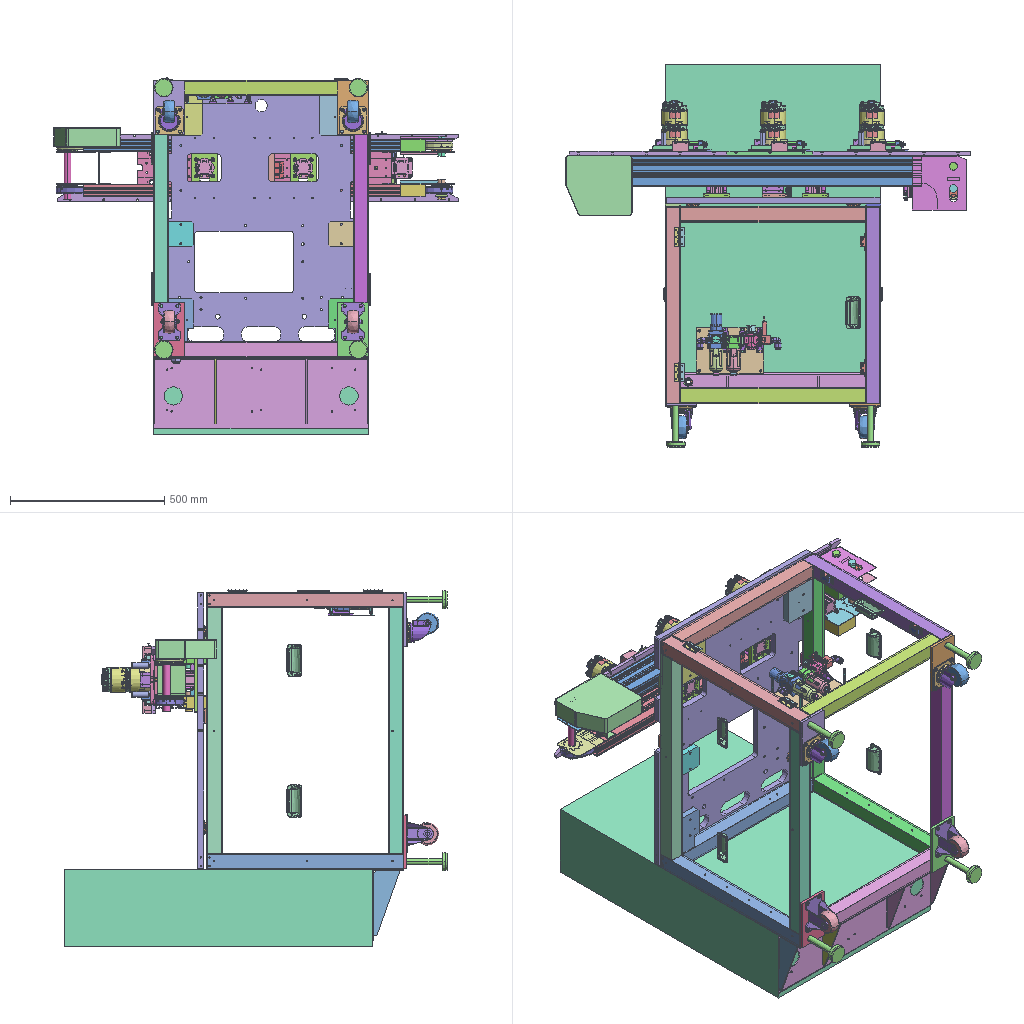Assembly | STEP file | 115 different items | 496 placed | box 1312 x 1242 x 1158 mm
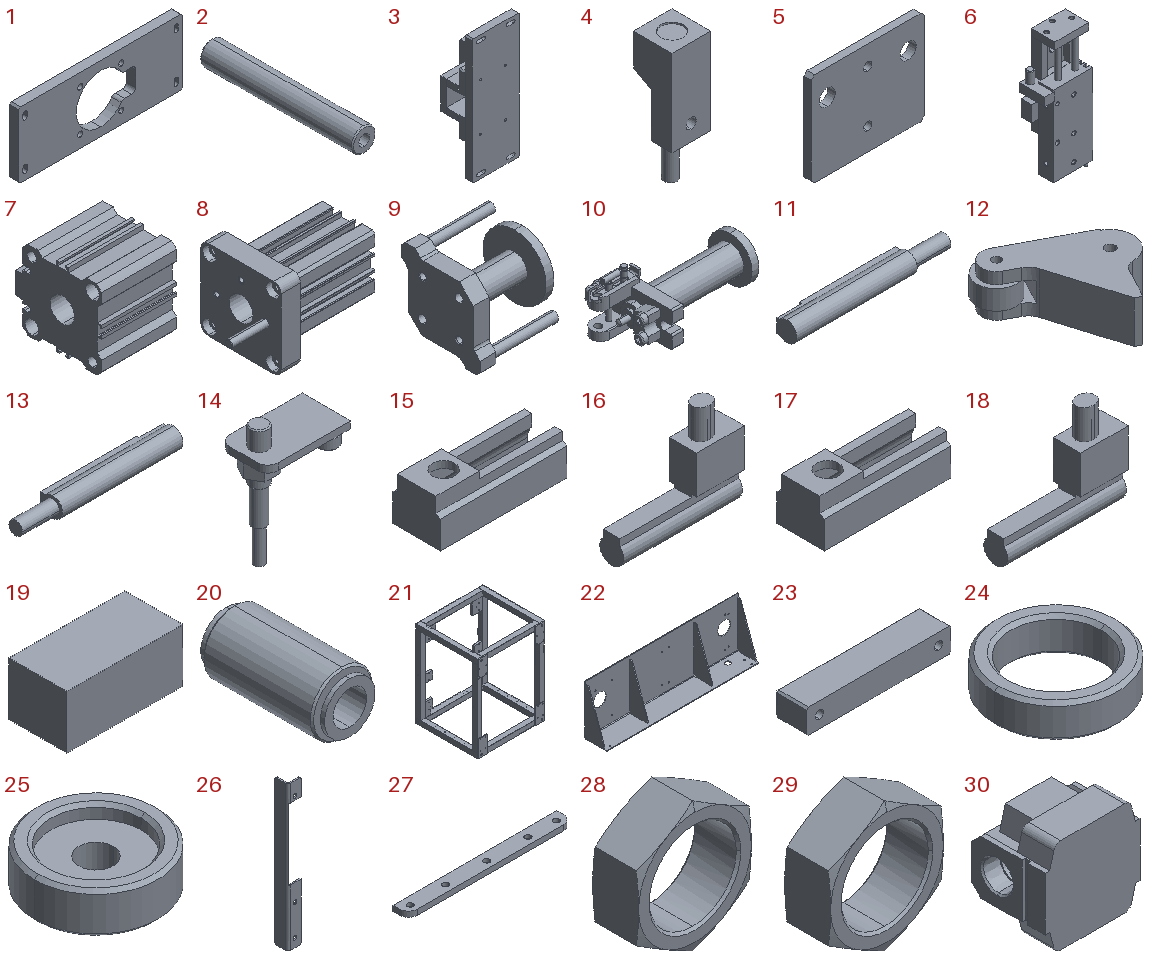Parts list (item | name | quantity | parent item | size | volume):
1 | 1105-104P042 | x2 | in 1105 brake cylinder | 211 x 12 x 85 mm | 165704 mm3
2 | 1105-104P043 | x12 | in 1105 brake cylinder | 11 x 71 x 11 mm | 6130 mm3
3 | 1105-104P044 | x1 | in 1105WWTCDQMB40-10-A93L_0_0_0_ | 79.5 x 92 x 211 mm | 345527 mm3
4 | 1105WWAAPS4-12M-Z-R-1-001 | x3 | in PN_0002 in-position detection Default | 12 x 12 x 37 mm | 2919 mm3
5 | 1105WWASensor BKT | x3 | in PN_0002 in-position detection Default | 35 x 2.3 x 29 mm | 2217 mm3
6 | 1105WWMXQ12-40CSP-M9NL(35)527 | x1 | in 1105WWNACCTV松Product-00527 | 56.1 x 30 x 145 mm | 123315 mm3
7 | 1105WWT1_1 | x1 | in 1105WWTCDQMB40-10-A93L_0_0_0_ | 49.5 x 57 x 52 mm | 94485 mm3
8 | 1105WWT1_2 | x3 | - | 120 x 67 x 67 mm | 176582 mm3
9 | 1105WWT2_1 | x1 | in 1105WWTCDQMB40-10-A93L_0_0_0_ | 51.75 x 50 x 50 mm | 33168 mm3
10 | 1105WWT2_2 | x3 | - | 97 x 42.5 x 39.25 mm | 37426 mm3
11 | 1105WWT3 | x1 | in 1105WWTCDQMB40-10-A93L_0_0_0_ | 32 x 4.5 x 4 mm | 389.357 mm3
12 | 1105WWT3_1 | x3 | - | 33.665 x 38.307 x 13 mm | 6665 mm3
13 | 1105WWT4 | x1 | in 1105WWTCDQMB40-10-A93L_0_0_0_ | 32 x 4.5 x 4 mm | 389.357 mm3
14 | 1105WWT4_1 | x3 | - | 24.119 x 14.25 x 35 mm | 1315 mm3
15 | 1105WWT5_1 | x3 | - | 16.5 x 6.2 x 5.9 mm | 230.408 mm3
16 | 1105WWT6_1 | x3 | - | 20 x 4.6 x 16.5 mm | 577.001 mm3
17 | 1105WWT7_1 | x3 | - | 16.5 x 6.2 x 5.9 mm | 230.408 mm3
18 | 1105WWT8_1 | x3 | - | 20 x 4.6 x 16.5 mm | 577.001 mm3
19 | 1105WW撞块-002_デフォルト | x3 | in 1105WW442_デフォルト | 30 x 15 x 13.8 mm | 6210 mm3
20 | 1_4 | x1 | in KQ2E12-00 | 22 x 44 x 22 mm | 10940 mm3
21 | 227H056111 Footstool Default | x1 | in 18 | 700 x 656 x 900 mm | 6881693 mm3
22 | 227H056114 BKT Default | x1 | in 18 | 700 x 100 x 230 mm | 887594 mm3
23 | 229H151426 Default | x6 | in PN_0018 Default | 80 x 17.5 x 13.5 mm | 17874 mm3
24 | 229H151427 Default | x6 | in PN_0018 Default | 18 x 18 x 5 mm | 563.602 mm3
25 | 229H151428 Default | x6 | in PN_0018 Default | 18 x 18 x 6 mm | 1155 mm3
26 | 229H151431 Default | x3 | in PN_0018 Default | 15 x 15 x 165 mm | 5074 mm3
27 | 229H151433 Default | x3 | in PN_0018 Default | 185 x 17.5 x 6 mm | 18413 mm3
28 | 2_4 | x1 | in KQ2E12-00 | 27 x 11 x 31.177 mm | 3125 mm3
29 | 3 | x1 | in KQ2E12-00 | 27 x 11 x 31.177 mm | 3125 mm3
30 | AFM30-03_AFM3022A Body_30 | x1 | in AFM30-03_AFM30-03 | 53 x 41 x 53 mm | 82463 mm3
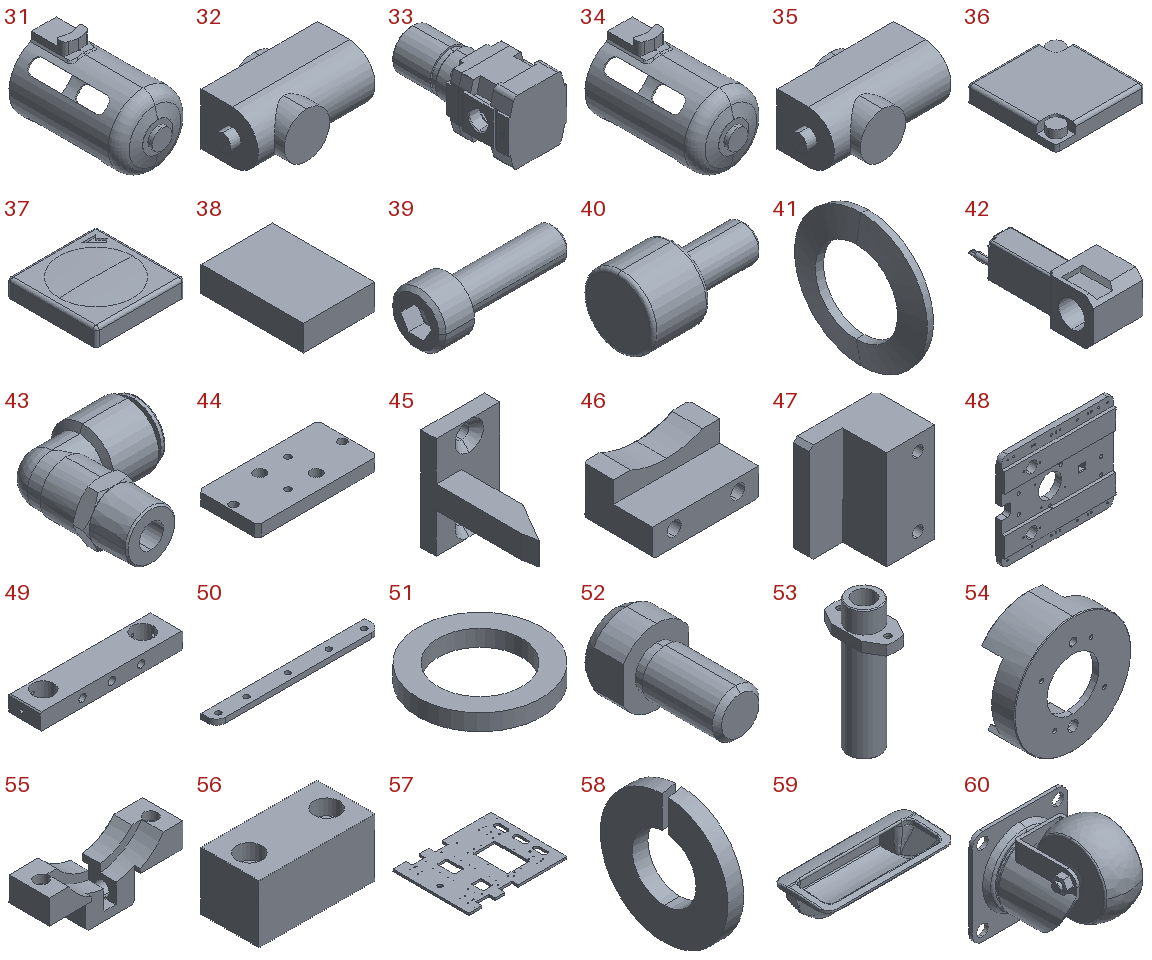31 | AFM30-03_AFM3022A Bowl_30 | x1 | in AFM30-03_AFM3022A Bowl Assy_30 | 45.5 x 76.9 x 53.25 mm | 11501 mm3
32 | AFM30-03_AFM3022A Drain_30 | x1 | in AFM30-03_AFM3022A Bowl Assy_30 | 19.5 x 11.1 x 8 mm | 1266 mm3
33 | AW30-03E_AW3020A Body_30 | x1 | in AW30-03E_AW30-03E | 53 x 113 x 57 mm | 188440 mm3
34 | AW30-03E_AW3020A Bowl_30 | x1 | in AW30-03E_AW3020A Bowl Assy_30 | 45.5 x 76.9 x 53.25 mm | 11501 mm3
35 | AW30-03E_AW3020A Drain_30 | x1 | in AW30-03E_AW3020A Bowl Assy_30 | 19.5 x 11.1 x 8 mm | 1266 mm3
36 | AW30-03E_AW3020A Gauge_30 | x1 | in AW30-03E_AW30-03E | 28 x 28 x 5.1 mm | 3850 mm3
37 | AW30-03E_AW3020A Gauge_30-E | x1 | in AW30-03E_AW30-03E | 28 x 28 x 5.8 mm | 4343 mm3
38 | BOX111 Default | x1 | in 18 | 700 x 1000 x 250 mm | 175000000 mm3
39 | CB6-20_デフォルト | x24 | in CB6-20_CW6_デフォルト, CB6-20_SW6_W6_デフォルト | 26 x 10 x 10 mm | 957.413 mm3
40 | CFFANG5-10_デフォルト | x3 | in PN_0018 Default | 18 x 10 x 10 mm | 819.54 mm3
41 | CW6 Default | x12 | in CB6-20_CW6_デフォルト | 0.95 x 10.5 x 10.5 mm | 31.798 mm3
42 | IS1000E-3003-X202_IS1000E3035GA Body_30 | x1 | in IS1000E-3003-X202_IS1000E-3003-X202 | 32 x 90.5 x 30 mm | 34770 mm3
43 | KQ2L12-03S_KQ2L_12-03 | x2 | in KQ2L12-03S_KQ2L12-03S | 38.315 x 43.45 x 20.9 mm | 10699 mm3
44 | PN_0002 top plate Default | x1 | in 1105WWTCDQMB40-10-A93L_0_0_0_ | 100 x 50 x 10 mm | 47660 mm3
45 | PN_0002NACCTV wedge pin 527 | x1 | in 1105WWNACCTV松Product-00527 | 25 x 45.321 x 40 mm | 8429 mm3
46 | PN_0004 Default | x3 | in PN_0018 Default | 50 x 33 x 23 mm | 24275 mm3
47 | PN_0006 Default | x9 | in PN_0018 Default | 41.5 x 29.8 x 50 mm | 40902 mm3
48 | PN_0007 Default | x3 | in PN_0018 Default | 185 x 15 x 160 mm | 319731 mm3
49 | PN_0008 Default | x3 | in PN_0018 Default | 129 x 29.5 x 15 mm | 43870 mm3
50 | PN_0009 Default | x3 | in PN_0018 Default | 185 x 17.5 x 6 mm | 18511 mm3
51 | PN_0010 Default | x3 | in PN_0018 Default | 7.5 x 7.5 x 1 mm | 23.75 mm3
52 | PN_0011 Default | x3 | in PN_0018 Default | 7 x 13.2 x 8 mm | 366.094 mm3
53 | PN_0016 Default | x6 | in PN_0018 Default | 20 x 36 x 72.5 mm | 11823 mm3
54 | PN_0017 Default | x3 | in PN_0018 Default | 90 x 34.5 x 90 mm | 46936 mm3
55 | PN_0019 Default | x3 | in PN_0018 Default | 110 x 33 x 44 mm | 53876 mm3
56 | PN_0020 Default | x9 | in PN_0018 Default | 30 x 15 x 15 mm | 6285 mm3
57 | PN_0022 Base Default | x1 | in 18 | 900 x 700 x 20 mm | 9845455 mm3
58 | SW6 Default | x12 | in CB6-20_SW6_W6_デフォルト | 1.5 x 12.2 x 12.197 mm | 128.674 mm3
59 | - | x5 | in 18 | 104 x 48 x 25.005 mm | 18990 mm3
60 | SceondCJH75 | x2 | in 18 | - | -
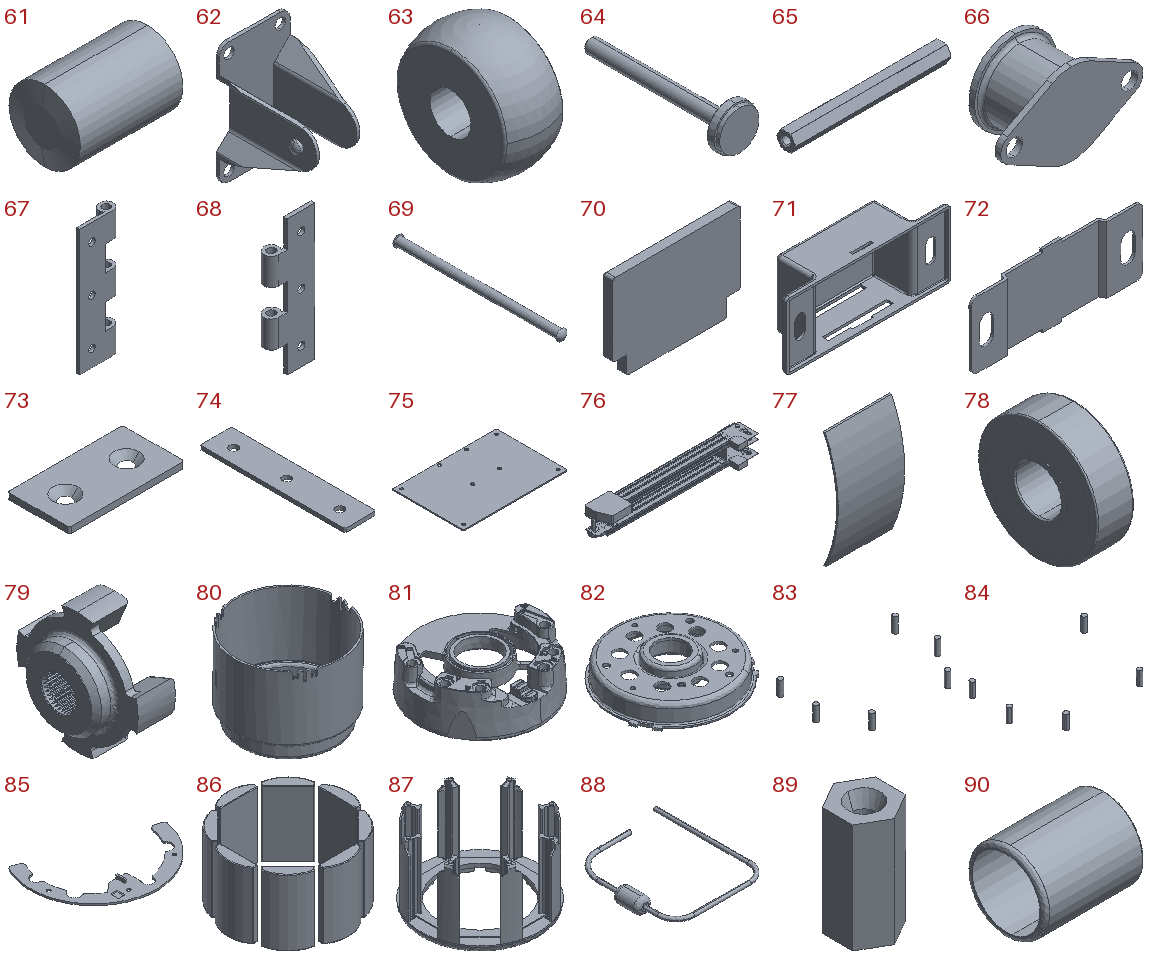61 | SceondCKH75bearing | x2 | in SceondCKH75 | 38 x 25 x 25 mm | 18231 mm3
62 | SceondCKH75fixed | x2 | in SceondCKH75 | 72 x 88.179 x 123 mm | 53019 mm3
63 | SceondCKH75wheel | x2 | in SceondCKH75 | 36 x 75 x 75 mm | 129056 mm3
64 | SceondD-B3-20-180 | x4 | in 18 | 60.3 x 210 x 60.3 mm | 105197 mm3
65 | SceondLSFB8-75 | x4 | in 18 | 75 x 9.2 x 8 mm | 3839 mm3
66 | SceondRB-45 | x4 | in 18 | 78 x 34 x 45 mm | 42765 mm3
67 | Second B-1027-14 Pin A Part | x2 | in SceondB-1027-14 | 19.25 x 6.5 x 60 mm | 2015 mm3
68 | Second B-1027-14 Pin B Part | x2 | in SceondB-1027-14 | 19.25 x 6.5 x 60 mm | 1700 mm3
69 | Second B-1027-14 Shaft Part | x2 | in SceondB-1027-14 | 4 x 62.171 x 4 mm | 439.342 mm3
70 | Second C-100-B Work Part | x2 | in 70 | 28 x 2 x 20 mm | 1071 mm3
71 | Second C-100-B-2 Base Part | x2 | in SceondC-100-B-2 | 56.5 x 15.3 x 23 mm | 2154 mm3
72 | Second C-100-B-2 Bracket Part | x2 | in SceondC-100-B-2 | 54.5 x 2.5 x 23 mm | 897.584 mm3
73 | Second C-100-B-2 Bracket Part [2] | x2 | in 18 | 30 x 16 x 1.6 mm | 705.168 mm3
74 | Second Door Spacer PN_0025 Default | x2 | in 18 | 13 x 60 x 1.6 mm | 1201 mm3
75 | Second M80U005006A Air System BKT Default | x1 | in 18 | 220 x 150 x 2.3 mm | 75278 mm3
76 | TCSW62A-MD-145-1213-18-90W-3-SC-1014_no bracket 2090<machined> | x1 | in Tshusongxian-01_デフォルト | 1300 x 197.8 x 232.2 mm | 4651494 mm3
77 | TQ-DD-1020-BIAOQIAN-001010 | x6 | in TQ-DD-1105-TH140P_HP_K04502_MotorAssy1010_デフォルト | 20 x 4.519 x 35 mm | 361.459 mm3
78 | TQ-DD-1105-TH 6000ZZ_2_031010 Default | x6 | in TQ-DD-1105-THRotorAssy1010_デフォルト | 8 x 26 x 26 mm | 2409 mm3
79 | TQ-DD-1105-TH SAP_405441541010 Default | x6 | in TQ-DD-1105-TH140P_HP_K04502_MotorAssy1010_デフォルト | 13.9 x 30 x 30 mm | 3137 mm3
80 | TQ-DD-1105-THA140062100B_Housing1010_デフォルト | x6 | in TQ-DD-1105-THHousingAssy1010_デフォルト | 82 x 82 x 64.1 mm | 27832 mm3
81 | TQ-DD-1105-THA160078900_Mold1010_デフォルト | x6 | in TQ-DD-1105-THTerminalAssy1010_デフォルト | 79.236 x 78.917 x 27.1 mm | 21027 mm3
82 | TQ-DD-1105-THBrg.Holder(A140059500A)1010_デフォルト | x6 | in TQ-DD-1105-THBrg.HolderAssy1010_デフォルト | 79.4 x 80.57 x 17.1 mm | 12458 mm3
83 | TQ-DD-1105-THCoil1010_デフォルト | x6 | in TQ-DD-1105-THStatorAssy31010_デフォルト | 46.175 x 30.321 x 5.639 mm | 82.319 mm3
84 | TQ-DD-1105-THCoil21010_デフォルト | x6 | in TQ-DD-1105-THStatorAssy31010_デフォルト | 48.573 x 32.204 x 5.639 mm | 77.064 mm3
85 | TQ-DD-1105-THCover1010_デフォルト | x6 | in TQ-DD-1105-THTerminalAssy1010_デフォルト | 73.74 x 54.492 x 3 mm | 881.003 mm3
86 | TQ-DD-1105-THMagnet1010_デフォルト | x12 | in TQ-DD-1105-THRotorCoreAssy1010_デフォルト | 39 x 39 x 21.5 mm | 6144 mm3
87 | TQ-DD-1105-THMagnetHolder1010_デフォルト | x12 | in TQ-DD-1105-THRotor1010_デフォルト | 38.83 x 38.83 x 24.45 mm | 2757 mm3
88 | TQ-DD-1105-THNTC Thermistor1010_デフォルト | x6 | in TQ-DD-1105-THTerminalAssy1010_デフォルト | 11.725 x 13.225 x 1.8 mm | 12.894 mm3
89 | TQ-DD-1105-THNuts1010_デフォルト | x36 | in TQ-DD-1105-THTerminalAssy1010_デフォルト | 6 x 6.928 x 12.4 mm | 316.696 mm3
90 | TQ-DD-1105-THRotor cover1010_デフォルト | x6 | in TQ-DD-1105-THRotorCoreAssy1010_デフォルト | 48.9 x 39.4 x 39.4 mm | 1331 mm3
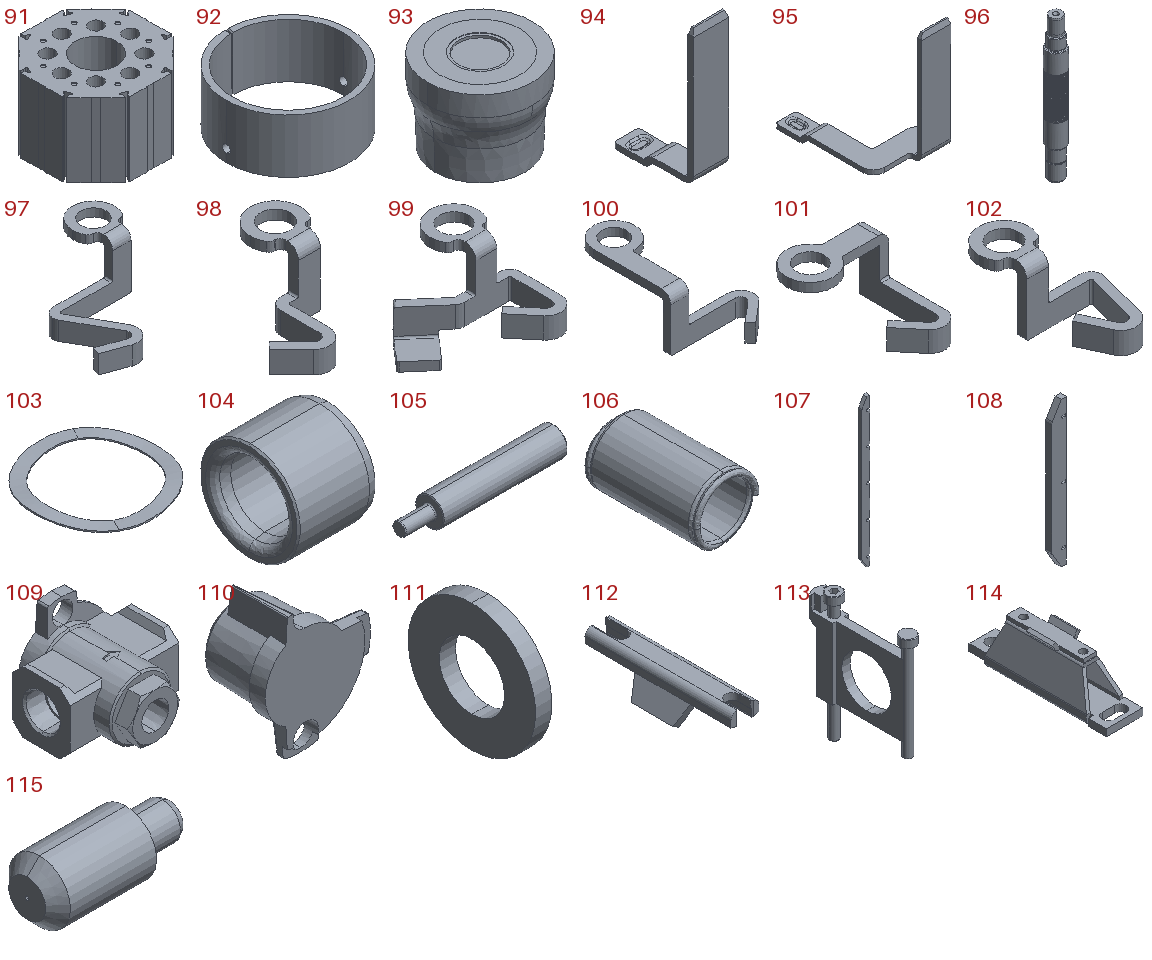91 | TQ-DD-1105-THRotorCore1010_デフォルト | x12 | in TQ-DD-1105-THRotor1010_デフォルト | 31.8 x 31.8 x 21.5 mm | 12871 mm3
92 | TQ-DD-1105-THSHIELD1010_デフォルト | x6 | in TQ-DD-1105-THTerminalAssy1010_デフォルト | 31 x 30.999 x 13.6 mm | 1876 mm3
93 | TQ-DD-1105-THSensorMagnet1010_デフォルト | x6 | in TQ-DD-1105-TH140P_HP_K04502_MotorAssy1010_デフォルト | 21 x 21 x 16.3 mm | 3743 mm3
94 | TQ-DD-1105-THSensorTerminalA1010_デフォルト | x6 | in TQ-DD-1105-THTerminalAssy1010_デフォルト | 4 x 9 x 16.36 mm | 51.218 mm3
95 | TQ-DD-1105-THSensorTerminalB1010_デフォルト | x6 | in TQ-DD-1105-THTerminalAssy1010_デフォルト | 9 x 15 x 16.36 mm | 71.439 mm3
96 | TQ-DD-1105-THShaft1010_デフォルト | x6 | in TQ-DD-1105-THShaftAssy1010_デフォルト | 12.206 x 12.206 x 96.2 mm | 9184 mm3
97 | TQ-DD-1105-THTerminalA1010_デフォルト | x6 | in TQ-DD-1105-THTerminalAssy1010_デフォルト | 18.96 x 21.767 x 10.4 mm | 259.607 mm3
98 | TQ-DD-1105-THTerminalB1010_デフォルト | x6 | in TQ-DD-1105-THTerminalAssy1010_デフォルト | 15.207 x 18.483 x 10.4 mm | 194.982 mm3
99 | TQ-DD-1105-THTerminalC1010_デフォルト | x6 | in TQ-DD-1105-THTerminalAssy1010_デフォルト | 18.722 x 18.871 x 12.9 mm | 306.798 mm3
100 | TQ-DD-1105-THTerminalD1010_デフォルト | x6 | in TQ-DD-1105-THTerminalAssy1010_デフォルト | 15.02 x 25.091 x 10.4 mm | 251.396 mm3
101 | TQ-DD-1105-THTerminalE1010_デフォルト | x6 | in TQ-DD-1105-THTerminalAssy1010_デフォルト | 15.586 x 17.763 x 10.4 mm | 231.793 mm3
102 | TQ-DD-1105-THTerminalF1010_デフォルト | x6 | in TQ-DD-1105-THTerminalAssy1010_デフォルト | 14.108 x 19.733 x 10.4 mm | 233.484 mm3
103 | TQ-DD-1105-THWWasher1010_デフォルト | x6 | in TQ-DD-1105-TH140P_HP_K04502_MotorAssy1010_デフォルト | 24.801 x 24.797 x 1.007 mm | 43.898 mm3
104 | TQ-DD-1105WWmpbz13_15_2_031010 | x3 | in PN_0018 Default | 15 x 19 x 19 mm | 2146 mm3
105 | TQ-DD-AAsfad13_65_f12_b7_p6_n6_2_031010 | x6 | in PN_0018 Default | 71 x 13 x 13 mm | 7610 mm3
106 | TQ-DD-ul20_35_2_031010 | x6 | in PN_0018 Default | 20 x 35 x 20 mm | 3226 mm3
107 | Tdangtiao-001_デフォルト | x4 | in Tshusongxian-01_デフォルト | 28 x 12 x 510.5 mm | 161527 mm3
108 | Tdangtiao-002_デフォルト | x2 | in Tshusongxian-01_デフォルト | 28 x 12 x 280 mm | 85542 mm3
109 | VHS30-03_VHS3035BA Body_30 | x1 | in VHS30-03_VHS30-03 | 53 x 50.6 x 55 mm | 43181 mm3
110 | VHS30-03_VHS3035BA Handle_30 | x1 | in VHS30-03_VHS30-03 | 43.43 x 27.4 x 50.43 mm | 21299 mm3
111 | W6 Default | x12 | in CB6-20_SW6_W6_デフォルト | 1.6 x 12.5 x 12.5 mm | 144.878 mm3
112 | Y300T_Y3035DB Front Plate_3 | x3 | in Y300T_Y300T | 14.986 x 44.8 x 10.145 mm | 1347 mm3
113 | Y300T_Y3035DB Interface_3 | x3 | in Y300T_Y300T | 7.2 x 46.6 x 59 mm | 5410 mm3
114 | Y300T_Y3035DB Rear Plate_3T | x3 | in Y300T_Y300T | 21 x 82 x 28.179 mm | 11258 mm3
115 | kfsaph5_p2_90_l8_b3_0_e0_5_a30_2_03 | x3 | in PN_0018 Default | 11.5 x 5 x 5 mm | 172.579 mm3